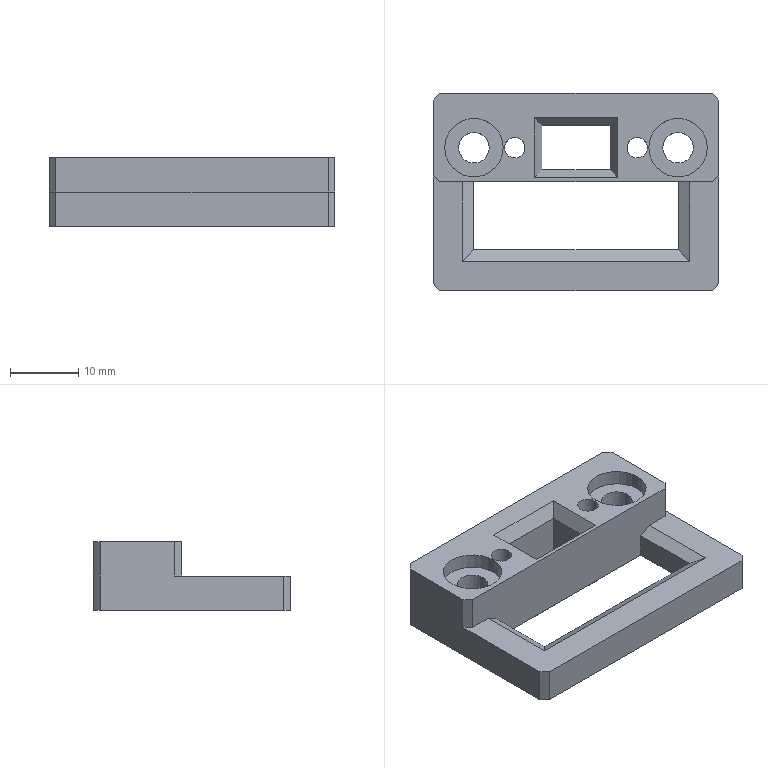Part | NX | features BREP 1 | 1 solid | 50 faces | box 42 x 29 x 10 mm | volume 5876 mm3 | plane 38 | cylinder 12 | commonest cylinder face diameters 3 x4 4.5 x4 8.6 x4
STEP:
#1=CARTESIAN_POINT('',(7.5,0.,-10.));
#2=VERTEX_POINT('',#1);
#3=CARTESIAN_POINT('',(10.5,0.,-10.));
#4=VERTEX_POINT('',#3);
#5=CARTESIAN_POINT('',(9.,0.,-10.));
#6=DIRECTION('',(0.,0.,1.));
#7=DIRECTION('',(1.,0.,0.));
#8=AXIS2_PLACEMENT_3D('',#5,#6,#7);
#9=CIRCLE('',#8,1.5);
#10=EDGE_CURVE('',#2,#4,#9,.T.);
#11=ORIENTED_EDGE('',*,*,#10,.F.);
#12=CARTESIAN_POINT('',(7.5,0.,0.));
#13=VERTEX_POINT('',#12);
#14=CARTESIAN_POINT('',(7.5,0.,-19.));
#15=DIRECTION('',(0.,0.,1.));
#16=VECTOR('',#15,1000.);
#17=LINE('',#14,#16);
#18=EDGE_CURVE('',#13,#2,#17,.F.);
#19=ORIENTED_EDGE('',*,*,#18,.F.);
#20=CARTESIAN_POINT('',(10.5,0.,0.));
#21=VERTEX_POINT('',#20);
#22=CARTESIAN_POINT('',(9.,0.,0.));
#23=DIRECTION('',(0.,0.,1.));
#24=DIRECTION('',(1.,0.,0.));
#25=AXIS2_PLACEMENT_3D('',#22,#23,#24);
#26=CIRCLE('',#25,1.5);
#27=EDGE_CURVE('',#13,#21,#26,.T.);
#28=ORIENTED_EDGE('',*,*,#27,.T.);
#29=CARTESIAN_POINT('',(10.5,0.,-19.));
#30=DIRECTION('',(0.,0.,1.));
#31=VECTOR('',#30,1000.);
#32=LINE('',#29,#31);
#33=EDGE_CURVE('',#21,#4,#32,.F.);
#34=ORIENTED_EDGE('',*,*,#33,.T.);
#35=EDGE_LOOP('',(#11,#19,#28,#34));
#36=FACE_BOUND('',#35,.T.);
#37=CARTESIAN_POINT('',(9.,0.,-19.));
#38=DIRECTION('',(0.,0.,1.));
#39=DIRECTION('',(1.,0.,0.));
#40=AXIS2_PLACEMENT_3D('',#37,#38,#39);
#41=CYLINDRICAL_SURFACE('',#40,1.5);
#42=ADVANCED_FACE('',(#36),#41,.F.);
#43=CARTESIAN_POINT('',(-10.5,0.,-10.));
#44=VERTEX_POINT('',#43);
#45=CARTESIAN_POINT('',(-7.5,0.,-10.));
#46=VERTEX_POINT('',#45);
#47=CARTESIAN_POINT('',(-9.,0.,-10.));
#48=DIRECTION('',(0.,0.,1.));
#49=DIRECTION('',(1.,0.,0.));
#50=AXIS2_PLACEMENT_3D('',#47,#48,#49);
#51=CIRCLE('',#50,1.5);
#52=EDGE_CURVE('',#44,#46,#51,.T.);
#53=ORIENTED_EDGE('',*,*,#52,.F.);
#54=CARTESIAN_POINT('',(-10.5,0.,0.));
#55=VERTEX_POINT('',#54);
#56=CARTESIAN_POINT('',(-10.5,0.,-19.));
#57=DIRECTION('',(0.,0.,1.));
#58=VECTOR('',#57,1000.);
#59=LINE('',#56,#58);
#60=EDGE_CURVE('',#55,#44,#59,.F.);
#61=ORIENTED_EDGE('',*,*,#60,.F.);
#62=CARTESIAN_POINT('',(-7.5,0.,0.));
#63=VERTEX_POINT('',#62);
#64=CARTESIAN_POINT('',(-9.,0.,0.));
#65=DIRECTION('',(0.,0.,1.));
#66=DIRECTION('',(1.,0.,0.));
#67=AXIS2_PLACEMENT_3D('',#64,#65,#66);
#68=CIRCLE('',#67,1.5);
#69=EDGE_CURVE('',#55,#63,#68,.T.);
#70=ORIENTED_EDGE('',*,*,#69,.T.);
#71=CARTESIAN_POINT('',(-7.5,0.,-19.));
#72=DIRECTION('',(0.,0.,1.));
#73=VECTOR('',#72,1000.);
#74=LINE('',#71,#73);
#75=EDGE_CURVE('',#63,#46,#74,.F.);
#76=ORIENTED_EDGE('',*,*,#75,.T.);
#77=EDGE_LOOP('',(#53,#61,#70,#76));
#78=FACE_BOUND('',#77,.T.);
#79=CARTESIAN_POINT('',(-9.,0.,-19.));
#80=DIRECTION('',(0.,0.,1.));
#81=DIRECTION('',(1.,0.,0.));
#82=AXIS2_PLACEMENT_3D('',#79,#80,#81);
#83=CYLINDRICAL_SURFACE('',#82,1.5);
#84=ADVANCED_FACE('',(#78),#83,.F.);
#85=CARTESIAN_POINT('',(-19.3,0.,-2.2));
#86=VERTEX_POINT('',#85);
#87=CARTESIAN_POINT('',(-10.7,0.,-2.2));
#88=VERTEX_POINT('',#87);
#89=CARTESIAN_POINT('',(-15.,0.,-2.2));
#90=DIRECTION('',(0.,0.,1.));
#91=DIRECTION('',(1.,0.,0.));
#92=AXIS2_PLACEMENT_3D('',#89,#90,#91);
#93=CIRCLE('',#92,4.3);
#94=EDGE_CURVE('',#86,#88,#93,.T.);
#95=ORIENTED_EDGE('',*,*,#94,.F.);
#96=CARTESIAN_POINT('',(-19.3,0.,0.));
#97=VERTEX_POINT('',#96);
#98=CARTESIAN_POINT('',(-19.3,0.,0.));
#99=DIRECTION('',(0.,0.,1.));
#100=VECTOR('',#99,1000.);
#101=LINE('',#98,#100);
#102=EDGE_CURVE('',#97,#86,#101,.F.);
#103=ORIENTED_EDGE('',*,*,#102,.F.);
#104=CARTESIAN_POINT('',(-10.7,0.,0.));
#105=VERTEX_POINT('',#104);
#106=CARTESIAN_POINT('',(-15.,0.,0.));
#107=DIRECTION('',(0.,0.,1.));
#108=DIRECTION('',(1.,0.,0.));
#109=AXIS2_PLACEMENT_3D('',#106,#107,#108);
#110=CIRCLE('',#109,4.3);
#111=EDGE_CURVE('',#97,#105,#110,.T.);
#112=ORIENTED_EDGE('',*,*,#111,.T.);
#113=CARTESIAN_POINT('',(-10.7,0.,0.));
#114=DIRECTION('',(0.,0.,1.));
#115=VECTOR('',#114,1000.);
#116=LINE('',#113,#115);
#117=EDGE_CURVE('',#105,#88,#116,.F.);
#118=ORIENTED_EDGE('',*,*,#117,.T.);
#119=EDGE_LOOP('',(#95,#103,#112,#118));
#120=FACE_BOUND('',#119,.T.);
#121=CARTESIAN_POINT('',(-15.,0.,0.));
#122=DIRECTION('',(0.,0.,1.));
#123=DIRECTION('',(1.,0.,0.));
#124=AXIS2_PLACEMENT_3D('',#121,#122,#123);
#125=CYLINDRICAL_SURFACE('',#124,4.3);
#126=ADVANCED_FACE('',(#120),#125,.F.);
#127=CARTESIAN_POINT('',(-17.25,0.,-10.));
#128=VERTEX_POINT('',#127);
#129=CARTESIAN_POINT('',(-12.75,0.,-10.));
#130=VERTEX_POINT('',#129);
#131=CARTESIAN_POINT('',(-15.,0.,-10.));
#132=DIRECTION('',(0.,0.,1.));
#133=DIRECTION('',(1.,0.,0.));
#134=AXIS2_PLACEMENT_3D('',#131,#132,#133);
#135=CIRCLE('',#134,2.25);
#136=EDGE_CURVE('',#128,#130,#135,.T.);
#137=ORIENTED_EDGE('',*,*,#136,.F.);
#138=CARTESIAN_POINT('',(-17.25,0.,-2.2));
#139=VERTEX_POINT('',#138);
#140=CARTESIAN_POINT('',(-17.25,0.,0.));
#141=DIRECTION('',(0.,0.,1.));
#142=VECTOR('',#141,1000.);
#143=LINE('',#140,#142);
#144=EDGE_CURVE('',#139,#128,#143,.F.);
#145=ORIENTED_EDGE('',*,*,#144,.F.);
#146=CARTESIAN_POINT('',(-12.75,0.,-2.2));
#147=VERTEX_POINT('',#146);
#148=CARTESIAN_POINT('',(-15.,0.,-2.2));
#149=DIRECTION('',(0.,0.,1.));
#150=DIRECTION('',(1.,0.,0.));
#151=AXIS2_PLACEMENT_3D('',#148,#149,#150);
#152=CIRCLE('',#151,2.25);
#153=EDGE_CURVE('',#139,#147,#152,.T.);
#154=ORIENTED_EDGE('',*,*,#153,.T.);
#155=CARTESIAN_POINT('',(-12.75,0.,0.));
#156=DIRECTION('',(0.,0.,1.));
#157=VECTOR('',#156,1000.);
#158=LINE('',#155,#157);
#159=EDGE_CURVE('',#147,#130,#158,.F.);
#160=ORIENTED_EDGE('',*,*,#159,.T.);
#161=EDGE_LOOP('',(#137,#145,#154,#160));
#162=FACE_BOUND('',#161,.T.);
#163=CARTESIAN_POINT('',(-15.,0.,0.));
#164=DIRECTION('',(0.,0.,1.));
#165=DIRECTION('',(1.,0.,0.));
#166=AXIS2_PLACEMENT_3D('',#163,#164,#165);
#167=CYLINDRICAL_SURFACE('',#166,2.25);
#168=ADVANCED_FACE('',(#162),#167,.F.);
#169=CARTESIAN_POINT('',(10.7,0.,-2.2));
#170=VERTEX_POINT('',#169);
#171=CARTESIAN_POINT('',(19.3,0.,-2.2));
#172=VERTEX_POINT('',#171);
#173=CARTESIAN_POINT('',(15.,0.,-2.2));
#174=DIRECTION('',(0.,0.,1.));
#175=DIRECTION('',(1.,0.,0.));
#176=AXIS2_PLACEMENT_3D('',#173,#174,#175);
#177=CIRCLE('',#176,4.3);
#178=EDGE_CURVE('',#170,#172,#177,.T.);
#179=ORIENTED_EDGE('',*,*,#178,.F.);
#180=CARTESIAN_POINT('',(10.7,0.,0.));
#181=VERTEX_POINT('',#180);
#182=CARTESIAN_POINT('',(10.7,0.,0.));
#183=DIRECTION('',(0.,0.,1.));
#184=VECTOR('',#183,1000.);
#185=LINE('',#182,#184);
#186=EDGE_CURVE('',#181,#170,#185,.F.);
#187=ORIENTED_EDGE('',*,*,#186,.F.);
#188=CARTESIAN_POINT('',(19.3,0.,0.));
#189=VERTEX_POINT('',#188);
#190=CARTESIAN_POINT('',(15.,0.,0.));
#191=DIRECTION('',(0.,0.,1.));
#192=DIRECTION('',(1.,0.,0.));
#193=AXIS2_PLACEMENT_3D('',#190,#191,#192);
#194=CIRCLE('',#193,4.3);
#195=EDGE_CURVE('',#181,#189,#194,.T.);
#196=ORIENTED_EDGE('',*,*,#195,.T.);
#197=CARTESIAN_POINT('',(19.3,0.,0.));
#198=DIRECTION('',(0.,0.,1.));
#199=VECTOR('',#198,1000.);
#200=LINE('',#197,#199);
#201=EDGE_CURVE('',#189,#172,#200,.F.);
#202=ORIENTED_EDGE('',*,*,#201,.T.);
#203=EDGE_LOOP('',(#179,#187,#196,#202));
#204=FACE_BOUND('',#203,.T.);
#205=CARTESIAN_POINT('',(15.,0.,0.));
#206=DIRECTION('',(0.,0.,1.));
#207=DIRECTION('',(1.,0.,0.));
#208=AXIS2_PLACEMENT_3D('',#205,#206,#207);
#209=CYLINDRICAL_SURFACE('',#208,4.3);
#210=ADVANCED_FACE('',(#204),#209,.F.);
#211=CARTESIAN_POINT('',(12.75,0.,-10.));
#212=VERTEX_POINT('',#211);
#213=CARTESIAN_POINT('',(17.25,0.,-10.));
#214=VERTEX_POINT('',#213);
#215=CARTESIAN_POINT('',(15.,0.,-10.));
#216=DIRECTION('',(0.,0.,1.));
#217=DIRECTION('',(1.,0.,0.));
#218=AXIS2_PLACEMENT_3D('',#215,#216,#217);
#219=CIRCLE('',#218,2.25);
#220=EDGE_CURVE('',#212,#214,#219,.T.);
#221=ORIENTED_EDGE('',*,*,#220,.F.);
#222=CARTESIAN_POINT('',(12.75,0.,-2.2));
#223=VERTEX_POINT('',#222);
#224=CARTESIAN_POINT('',(12.75,0.,0.));
#225=DIRECTION('',(0.,0.,1.));
#226=VECTOR('',#225,1000.);
#227=LINE('',#224,#226);
#228=EDGE_CURVE('',#223,#212,#227,.F.);
#229=ORIENTED_EDGE('',*,*,#228,.F.);
#230=CARTESIAN_POINT('',(17.25,0.,-2.2));
#231=VERTEX_POINT('',#230);
#232=CARTESIAN_POINT('',(15.,0.,-2.2));
#233=DIRECTION('',(0.,0.,1.));
#234=DIRECTION('',(1.,0.,0.));
#235=AXIS2_PLACEMENT_3D('',#232,#233,#234);
#236=CIRCLE('',#235,2.25);
#237=EDGE_CURVE('',#223,#231,#236,.T.);
#238=ORIENTED_EDGE('',*,*,#237,.T.);
#239=CARTESIAN_POINT('',(17.25,0.,0.));
#240=DIRECTION('',(0.,0.,1.));
#241=VECTOR('',#240,1000.);
#242=LINE('',#239,#241);
#243=EDGE_CURVE('',#231,#214,#242,.F.);
#244=ORIENTED_EDGE('',*,*,#243,.T.);
#245=EDGE_LOOP('',(#221,#229,#238,#244));
#246=FACE_BOUND('',#245,.T.);
#247=CARTESIAN_POINT('',(15.,0.,0.));
#248=DIRECTION('',(0.,0.,1.));
#249=DIRECTION('',(1.,0.,0.));
#250=AXIS2_PLACEMENT_3D('',#247,#248,#249);
#251=CYLINDRICAL_SURFACE('',#250,2.25);
#252=ADVANCED_FACE('',(#246),#251,.F.);
#253=CARTESIAN_POINT('',(-20.,-21.,-5.));
#254=VERTEX_POINT('',#253);
#255=CARTESIAN_POINT('',(20.,-21.,-5.));
#256=VERTEX_POINT('',#255);
#257=CARTESIAN_POINT('',(-21.,-21.,-5.));
#258=DIRECTION('',(1.,0.,0.));
#259=VECTOR('',#258,1000.);
#260=LINE('',#257,#259);
#261=EDGE_CURVE('',#254,#256,#260,.T.);
#262=ORIENTED_EDGE('',*,*,#261,.F.);
#263=CARTESIAN_POINT('',(-20.,-21.,-10.));
#264=VERTEX_POINT('',#263);
#265=CARTESIAN_POINT('',(-20.,-21.,0.));
#266=DIRECTION('',(0.,0.,-1.));
#267=VECTOR('',#266,1000.);
#268=LINE('',#265,#267);
#269=EDGE_CURVE('',#254,#264,#268,.T.);
#270=ORIENTED_EDGE('',*,*,#269,.T.);
#271=CARTESIAN_POINT('',(20.,-21.,-10.));
#272=VERTEX_POINT('',#271);
#273=CARTESIAN_POINT('',(-21.,-21.,-10.));
#274=DIRECTION('',(1.,0.,0.));
#275=VECTOR('',#274,1000.);
#276=LINE('',#273,#275);
#277=EDGE_CURVE('',#264,#272,#276,.T.);
#278=ORIENTED_EDGE('',*,*,#277,.T.);
#279=CARTESIAN_POINT('',(20.,-21.,0.));
#280=DIRECTION('',(0.,0.,1.));
#281=VECTOR('',#280,1000.);
#282=LINE('',#279,#281);
#283=EDGE_CURVE('',#272,#256,#282,.T.);
#284=ORIENTED_EDGE('',*,*,#283,.T.);
#285=EDGE_LOOP('',(#262,#270,#278,#284));
#286=FACE_BOUND('',#285,.T.);
#287=CARTESIAN_POINT('',(0.,-21.,0.));
#288=DIRECTION('',(0.,-1.,0.));
#289=DIRECTION('',(0.,0.,-1.));
#290=AXIS2_PLACEMENT_3D('',#287,#288,#289);
#291=PLANE('',#290);
#292=ADVANCED_FACE('',(#286),#291,.T.);
#293=CARTESIAN_POINT('',(15.,-15.,-9.5));
#294=VERTEX_POINT('',#293);
#295=CARTESIAN_POINT('',(15.,-15.,-6.));
#296=VERTEX_POINT('',#295);
#297=CARTESIAN_POINT('',(15.,-15.,-16.));
#298=DIRECTION('',(0.,0.,1.));
#299=VECTOR('',#298,1000.);
#300=LINE('',#297,#299);
#301=EDGE_CURVE('',#294,#296,#300,.T.);
#302=ORIENTED_EDGE('',*,*,#301,.T.);
#303=CARTESIAN_POINT('',(15.,-5.,-6.));
#304=VERTEX_POINT('',#303);
#305=CARTESIAN_POINT('',(15.,-5.,-6.));
#306=DIRECTION('',(0.,1.,0.));
#307=VECTOR('',#306,1000.);
#308=LINE('',#305,#307);
#309=EDGE_CURVE('',#296,#304,#308,.T.);
#310=ORIENTED_EDGE('',*,*,#309,.T.);
#311=CARTESIAN_POINT('',(15.,-5.,-9.5));
#312=VERTEX_POINT('',#311);
#313=CARTESIAN_POINT('',(15.,-5.,-16.));
#314=DIRECTION('',(0.,0.,1.));
#315=VECTOR('',#314,1000.);
#316=LINE('',#313,#315);
#317=EDGE_CURVE('',#312,#304,#316,.T.);
#318=ORIENTED_EDGE('',*,*,#317,.F.);
#319=CARTESIAN_POINT('',(15.,-15.,-9.5));
#320=DIRECTION('',(0.,-1.,0.));
#321=VECTOR('',#320,1000.);
#322=LINE('',#319,#321);
#323=EDGE_CURVE('',#312,#294,#322,.T.);
#324=ORIENTED_EDGE('',*,*,#323,.T.);
#325=EDGE_LOOP('',(#302,#310,#318,#324));
#326=FACE_BOUND('',#325,.T.);
#327=CARTESIAN_POINT('',(15.,-15.,-16.));
#328=DIRECTION('',(1.,0.,0.));
#329=DIRECTION('',(0.,1.,0.));
#330=AXIS2_PLACEMENT_3D('',#327,#328,#329);
#331=PLANE('',#330);
#332=ADVANCED_FACE('',(#326),#331,.F.);
#333=CARTESIAN_POINT('',(-15.,-15.,-9.5));
#334=VERTEX_POINT('',#333);
#335=CARTESIAN_POINT('',(-15.,-15.,-6.));
#336=VERTEX_POINT('',#335);
#337=CARTESIAN_POINT('',(-15.,-15.,-16.));
#338=DIRECTION('',(0.,0.,1.));
#339=VECTOR('',#338,1000.);
#340=LINE('',#337,#339);
#341=EDGE_CURVE('',#334,#336,#340,.T.);
#342=ORIENTED_EDGE('',*,*,#341,.T.);
#343=CARTESIAN_POINT('',(15.,-15.,-6.));
#344=DIRECTION('',(1.,0.,0.));
#345=VECTOR('',#344,1000.);
#346=LINE('',#343,#345);
#347=EDGE_CURVE('',#336,#296,#346,.T.);
#348=ORIENTED_EDGE('',*,*,#347,.T.);
#349=ORIENTED_EDGE('',*,*,#301,.F.);
#350=CARTESIAN_POINT('',(15.,-15.,-9.5));
#351=DIRECTION('',(-1.,0.,0.));
#352=VECTOR('',#351,1000.);
#353=LINE('',#350,#352);
#354=EDGE_CURVE('',#294,#334,#353,.T.);
#355=ORIENTED_EDGE('',*,*,#354,.T.);
#356=EDGE_LOOP('',(#342,#348,#349,#355));
#357=FACE_BOUND('',#356,.T.);
#358=CARTESIAN_POINT('',(15.,-15.,-16.));
#359=DIRECTION('',(0.,-1.,0.));
#360=DIRECTION('',(0.,0.,-1.));
#361=AXIS2_PLACEMENT_3D('',#358,#359,#360);
#362=PLANE('',#361);
#363=ADVANCED_FACE('',(#357),#362,.F.);
#364=CARTESIAN_POINT('',(-15.,-5.,-9.5));
#365=VERTEX_POINT('',#364);
#366=CARTESIAN_POINT('',(-15.,-5.,-6.));
#367=VERTEX_POINT('',#366);
#368=CARTESIAN_POINT('',(-15.,-5.,-16.));
#369=DIRECTION('',(0.,0.,1.));
#370=VECTOR('',#369,1000.);
#371=LINE('',#368,#370);
#372=EDGE_CURVE('',#365,#367,#371,.T.);
#373=ORIENTED_EDGE('',*,*,#372,.T.);
#374=CARTESIAN_POINT('',(-15.,-15.,-6.));
#375=DIRECTION('',(0.,-1.,0.));
#376=VECTOR('',#375,1000.);
#377=LINE('',#374,#376);
#378=EDGE_CURVE('',#367,#336,#377,.T.);
#379=ORIENTED_EDGE('',*,*,#378,.T.);
#380=ORIENTED_EDGE('',*,*,#341,.F.);
#381=CARTESIAN_POINT('',(-15.,-15.,-9.5));
#382=DIRECTION('',(0.,1.,0.));
#383=VECTOR('',#382,1000.);
#384=LINE('',#381,#383);
#385=EDGE_CURVE('',#334,#365,#384,.T.);
#386=ORIENTED_EDGE('',*,*,#385,.T.);
#387=EDGE_LOOP('',(#373,#379,#380,#386));
#388=FACE_BOUND('',#387,.T.);
#389=CARTESIAN_POINT('',(-15.,-15.,-16.));
#390=DIRECTION('',(-1.,0.,0.));
#391=DIRECTION('',(0.,0.,1.));
#392=AXIS2_PLACEMENT_3D('',#389,#390,#391);
#393=PLANE('',#392);
#394=ADVANCED_FACE('',(#388),#393,.F.);
#395=CARTESIAN_POINT('',(21.,-4.,0.));
#396=VERTEX_POINT('',#395);
#397=CARTESIAN_POINT('',(21.,7.,0.));
#398=VERTEX_POINT('',#397);
#399=CARTESIAN_POINT('',(21.,5.,0.));
#400=DIRECTION('',(0.,1.,0.));
#401=VECTOR('',#400,1000.);
#402=LINE('',#399,#401);
#403=EDGE_CURVE('',#396,#398,#402,.T.);
#404=ORIENTED_EDGE('',*,*,#403,.F.);
#405=CARTESIAN_POINT('',(21.,-4.,-5.));
#406=VERTEX_POINT('',#405);
#407=CARTESIAN_POINT('',(21.,-4.,-5.));
#408=DIRECTION('',(0.,0.,-1.));
#409=VECTOR('',#408,1000.);
#410=LINE('',#407,#409);
#411=EDGE_CURVE('',#396,#406,#410,.T.);
#412=ORIENTED_EDGE('',*,*,#411,.T.);
#413=CARTESIAN_POINT('',(21.,-20.,-5.));
#414=VERTEX_POINT('',#413);
#415=CARTESIAN_POINT('',(21.,-5.,-5.));
#416=DIRECTION('',(0.,1.,0.));
#417=VECTOR('',#416,1000.);
#418=LINE('',#415,#417);
#419=EDGE_CURVE('',#414,#406,#418,.T.);
#420=ORIENTED_EDGE('',*,*,#419,.F.);
#421=CARTESIAN_POINT('',(21.,-20.,-10.));
#422=VERTEX_POINT('',#421);
#423=CARTESIAN_POINT('',(21.,-20.,-10.));
#424=DIRECTION('',(0.,0.,-1.));
#425=VECTOR('',#424,1000.);
#426=LINE('',#423,#425);
#427=EDGE_CURVE('',#414,#422,#426,.T.);
#428=ORIENTED_EDGE('',*,*,#427,.T.);
#429=CARTESIAN_POINT('',(21.,7.,-10.));
#430=VERTEX_POINT('',#429);
#431=CARTESIAN_POINT('',(21.,5.,-10.));
#432=DIRECTION('',(0.,1.,0.));
#433=VECTOR('',#432,1000.);
#434=LINE('',#431,#433);
#435=EDGE_CURVE('',#422,#430,#434,.T.);
#436=ORIENTED_EDGE('',*,*,#435,.T.);
#437=CARTESIAN_POINT('',(21.,7.,-10.));
#438=DIRECTION('',(0.,0.,1.));
#439=VECTOR('',#438,1000.);
#440=LINE('',#437,#439);
#441=EDGE_CURVE('',#430,#398,#440,.T.);
#442=ORIENTED_EDGE('',*,*,#441,.T.);
#443=EDGE_LOOP('',(#404,#412,#420,#428,#436,#442));
#444=FACE_BOUND('',#443,.T.);
#445=CARTESIAN_POINT('',(21.,5.,-10.));
#446=DIRECTION('',(1.,0.,0.));
#447=DIRECTION('',(0.,1.,0.));
#448=AXIS2_PLACEMENT_3D('',#445,#446,#447);
#449=PLANE('',#448);
#450=ADVANCED_FACE('',(#444),#449,.T.);
#451=CARTESIAN_POINT('',(-21.,-4.,-5.));
#452=VERTEX_POINT('',#451);
#453=CARTESIAN_POINT('',(-21.,-20.,-5.));
#454=VERTEX_POINT('',#453);
#455=CARTESIAN_POINT('',(-21.,-5.,-5.));
#456=DIRECTION('',(0.,-1.,0.));
#457=VECTOR('',#456,1000.);
#458=LINE('',#455,#457);
#459=EDGE_CURVE('',#452,#454,#458,.T.);
#460=ORIENTED_EDGE('',*,*,#459,.F.);
#461=CARTESIAN_POINT('',(-21.,-4.,0.));
#462=VERTEX_POINT('',#461);
#463=CARTESIAN_POINT('',(-21.,-4.,0.));
#464=DIRECTION('',(0.,0.,1.));
#465=VECTOR('',#464,1000.);
#466=LINE('',#463,#465);
#467=EDGE_CURVE('',#452,#462,#466,.T.);
#468=ORIENTED_EDGE('',*,*,#467,.T.);
#469=CARTESIAN_POINT('',(-21.,7.,0.));
#470=VERTEX_POINT('',#469);
#471=CARTESIAN_POINT('',(-21.,5.,0.));
#472=DIRECTION('',(0.,-1.,0.));
#473=VECTOR('',#472,1000.);
#474=LINE('',#471,#473);
#475=EDGE_CURVE('',#470,#462,#474,.T.);
#476=ORIENTED_EDGE('',*,*,#475,.F.);
#477=CARTESIAN_POINT('',(-21.,7.,-10.));
#478=VERTEX_POINT('',#477);
#479=CARTESIAN_POINT('',(-21.,7.,-10.));
#480=DIRECTION('',(0.,0.,-1.));
#481=VECTOR('',#480,1000.);
#482=LINE('',#479,#481);
#483=EDGE_CURVE('',#470,#478,#482,.T.);
#484=ORIENTED_EDGE('',*,*,#483,.T.);
#485=CARTESIAN_POINT('',(-21.,-20.,-10.));
#486=VERTEX_POINT('',#485);
#487=CARTESIAN_POINT('',(-21.,5.,-10.));
#488=DIRECTION('',(0.,-1.,0.));
#489=VECTOR('',#488,1000.);
#490=LINE('',#487,#489);
#491=EDGE_CURVE('',#478,#486,#490,.T.);
#492=ORIENTED_EDGE('',*,*,#491,.T.);
#493=CARTESIAN_POINT('',(-21.,-20.,-10.));
#494=DIRECTION('',(0.,0.,1.));
#495=VECTOR('',#494,1000.);
#496=LINE('',#493,#495);
#497=EDGE_CURVE('',#486,#454,#496,.T.);
#498=ORIENTED_EDGE('',*,*,#497,.T.);
#499=EDGE_LOOP('',(#460,#468,#476,#484,#492,#498));
#500=FACE_BOUND('',#499,.T.);
#501=CARTESIAN_POINT('',(-21.,5.,-10.));
#502=DIRECTION('',(-1.,0.,0.));
#503=DIRECTION('',(0.,1.,0.));
#504=AXIS2_PLACEMENT_3D('',#501,#502,#503);
#505=PLANE('',#504);
#506=ADVANCED_FACE('',(#500),#505,.T.);
#507=ORIENTED_EDGE('',*,*,#277,.F.);
#508=CARTESIAN_POINT('',(-20.,-21.,-10.));
#509=DIRECTION('',(-0.7071,0.7071,0.));
#510=VECTOR('',#509,1000.);
#511=LINE('',#508,#510);
#512=EDGE_CURVE('',#264,#486,#511,.T.);
#513=ORIENTED_EDGE('',*,*,#512,.T.);
#514=ORIENTED_EDGE('',*,*,#491,.F.);
#515=CARTESIAN_POINT('',(-20.,8.,-10.));
#516=VERTEX_POINT('',#515);
#517=CARTESIAN_POINT('',(-20.,8.,-10.));
#518=DIRECTION('',(0.7071,0.7071,0.));
#519=VECTOR('',#518,1000.);
#520=LINE('',#517,#519);
#521=EDGE_CURVE('',#478,#516,#520,.T.);
#522=ORIENTED_EDGE('',*,*,#521,.T.);
#523=CARTESIAN_POINT('',(20.,8.,-10.));
#524=VERTEX_POINT('',#523);
#525=CARTESIAN_POINT('',(-21.,8.,-10.));
#526=DIRECTION('',(-1.,0.,0.));
#527=VECTOR('',#526,1000.);
#528=LINE('',#525,#527);
#529=EDGE_CURVE('',#524,#516,#528,.T.);
#530=ORIENTED_EDGE('',*,*,#529,.F.);
#531=CARTESIAN_POINT('',(20.,8.,-10.));
#532=DIRECTION('',(0.7071,-0.7071,0.));
#533=VECTOR('',#532,1000.);
#534=LINE('',#531,#533);
#535=EDGE_CURVE('',#524,#430,#534,.T.);
#536=ORIENTED_EDGE('',*,*,#535,.T.);
#537=ORIENTED_EDGE('',*,*,#435,.F.);
#538=CARTESIAN_POINT('',(20.,-21.,-10.));
#539=DIRECTION('',(-0.7071,-0.7071,0.));
#540=VECTOR('',#539,1000.);
#541=LINE('',#538,#540);
#542=EDGE_CURVE('',#422,#272,#541,.T.);
#543=ORIENTED_EDGE('',*,*,#542,.T.);
#544=EDGE_LOOP('',(#507,#513,#514,#522,#530,#536,#537,#543));
#545=FACE_BOUND('',#544,.T.);
#546=CARTESIAN_POINT('',(15.5,-4.5,-10.));
#547=VERTEX_POINT('',#546);
#548=CARTESIAN_POINT('',(6.732,-4.5,-10.));
#549=VERTEX_POINT('',#548);
#550=CARTESIAN_POINT('',(0.,-4.5,-10.));
#551=DIRECTION('',(-1.,0.,0.));
#552=VECTOR('',#551,1000.);
#553=LINE('',#550,#552);
#554=EDGE_CURVE('',#547,#549,#553,.T.);
#555=ORIENTED_EDGE('',*,*,#554,.T.);
#556=CARTESIAN_POINT('',(6.732,4.982,-10.));
#557=VERTEX_POINT('',#556);
#558=CARTESIAN_POINT('',(6.732,0.,-10.));
#559=DIRECTION('',(0.,1.,0.));
#560=VECTOR('',#559,1000.);
#561=LINE('',#558,#560);
#562=EDGE_CURVE('',#549,#557,#561,.T.);
#563=ORIENTED_EDGE('',*,*,#562,.T.);
#564=CARTESIAN_POINT('',(-6.732,4.982,-10.));
#565=VERTEX_POINT('',#564);
#566=CARTESIAN_POINT('',(0.,4.982,-10.));
#567=DIRECTION('',(-1.,0.,0.));
#568=VECTOR('',#567,1000.);
#569=LINE('',#566,#568);
#570=EDGE_CURVE('',#557,#565,#569,.T.);
#571=ORIENTED_EDGE('',*,*,#570,.T.);
#572=CARTESIAN_POINT('',(-6.732,-4.5,-10.));
#573=VERTEX_POINT('',#572);
#574=CARTESIAN_POINT('',(-6.732,0.,-10.));
#575=DIRECTION('',(0.,-1.,0.));
#576=VECTOR('',#575,1000.);
#577=LINE('',#574,#576);
#578=EDGE_CURVE('',#565,#573,#577,.T.);
#579=ORIENTED_EDGE('',*,*,#578,.T.);
#580=CARTESIAN_POINT('',(-15.5,-4.5,-10.));
#581=VERTEX_POINT('',#580);
#582=CARTESIAN_POINT('',(0.,-4.5,-10.));
#583=DIRECTION('',(-1.,0.,0.));
#584=VECTOR('',#583,1000.);
#585=LINE('',#582,#584);
#586=EDGE_CURVE('',#573,#581,#585,.T.);
#587=ORIENTED_EDGE('',*,*,#586,.T.);
#588=CARTESIAN_POINT('',(-15.5,-15.5,-10.));
#589=VERTEX_POINT('',#588);
#590=CARTESIAN_POINT('',(-15.5,0.,-10.));
#591=DIRECTION('',(0.,-1.,0.));
#592=VECTOR('',#591,1000.);
#593=LINE('',#590,#592);
#594=EDGE_CURVE('',#581,#589,#593,.T.);
#595=ORIENTED_EDGE('',*,*,#594,.T.);
#596=CARTESIAN_POINT('',(15.5,-15.5,-10.));
#597=VERTEX_POINT('',#596);
#598=CARTESIAN_POINT('',(0.,-15.5,-10.));
#599=DIRECTION('',(1.,0.,0.));
#600=VECTOR('',#599,1000.);
#601=LINE('',#598,#600);
#602=EDGE_CURVE('',#589,#597,#601,.T.);
#603=ORIENTED_EDGE('',*,*,#602,.T.);
#604=CARTESIAN_POINT('',(15.5,0.,-10.));
#605=DIRECTION('',(0.,1.,0.));
#606=VECTOR('',#605,1000.);
#607=LINE('',#604,#606);
#608=EDGE_CURVE('',#597,#547,#607,.T.);
#609=ORIENTED_EDGE('',*,*,#608,.T.);
#610=EDGE_LOOP('',(#555,#563,#571,#579,#587,#595,#603,#609));
#611=FACE_BOUND('',#610,.T.);
#612=CARTESIAN_POINT('',(9.,0.,-10.));
#613=DIRECTION('',(0.,0.,1.));
#614=DIRECTION('',(1.,0.,0.));
#615=AXIS2_PLACEMENT_3D('',#612,#613,#614);
#616=CIRCLE('',#615,1.5);
#617=EDGE_CURVE('',#4,#2,#616,.T.);
#618=ORIENTED_EDGE('',*,*,#617,.T.);
#619=ORIENTED_EDGE('',*,*,#10,.T.);
#620=EDGE_LOOP('',(#618,#619));
#621=FACE_BOUND('',#620,.T.);
#622=CARTESIAN_POINT('',(-9.,0.,-10.));
#623=DIRECTION('',(0.,0.,1.));
#624=DIRECTION('',(1.,0.,0.));
#625=AXIS2_PLACEMENT_3D('',#622,#623,#624);
#626=CIRCLE('',#625,1.5);
#627=EDGE_CURVE('',#46,#44,#626,.T.);
#628=ORIENTED_EDGE('',*,*,#627,.T.);
#629=ORIENTED_EDGE('',*,*,#52,.T.);
#630=EDGE_LOOP('',(#628,#629));
#631=FACE_BOUND('',#630,.T.);
#632=CARTESIAN_POINT('',(-15.,0.,-10.));
#633=DIRECTION('',(0.,0.,1.));
#634=DIRECTION('',(1.,0.,0.));
#635=AXIS2_PLACEMENT_3D('',#632,#633,#634);
#636=CIRCLE('',#635,2.25);
#637=EDGE_CURVE('',#130,#128,#636,.T.);
#638=ORIENTED_EDGE('',*,*,#637,.T.);
#639=ORIENTED_EDGE('',*,*,#136,.T.);
#640=EDGE_LOOP('',(#638,#639));
#641=FACE_BOUND('',#640,.T.);
#642=CARTESIAN_POINT('',(15.,0.,-10.));
#643=DIRECTION('',(0.,0.,1.));
#644=DIRECTION('',(1.,0.,0.));
#645=AXIS2_PLACEMENT_3D('',#642,#643,#644);
#646=CIRCLE('',#645,2.25);
#647=EDGE_CURVE('',#214,#212,#646,.T.);
#648=ORIENTED_EDGE('',*,*,#647,.T.);
#649=ORIENTED_EDGE('',*,*,#220,.T.);
#650=EDGE_LOOP('',(#648,#649));
#651=FACE_BOUND('',#650,.T.);
#652=CARTESIAN_POINT('',(0.,0.,-10.));
#653=DIRECTION('',(0.,0.,1.));
#654=DIRECTION('',(1.,0.,0.));
#655=AXIS2_PLACEMENT_3D('',#652,#653,#654);
#656=PLANE('',#655);
#657=ADVANCED_FACE('',(#545,#611,#621,#631,#641,#651),#656,.F.);
#658=ORIENTED_EDGE('',*,*,#475,.T.);
#659=CARTESIAN_POINT('',(-20.,-5.,0.));
#660=VERTEX_POINT('',#659);
#661=CARTESIAN_POINT('',(-12.5,-12.5,0.));
#662=DIRECTION('',(0.7071,-0.7071,0.));
#663=VECTOR('',#662,1000.);
#664=LINE('',#661,#663);
#665=EDGE_CURVE('',#462,#660,#664,.T.);
#666=ORIENTED_EDGE('',*,*,#665,.T.);
#667=CARTESIAN_POINT('',(20.,-5.,0.));
#668=VERTEX_POINT('',#667);
#669=CARTESIAN_POINT('',(15.,-5.,0.));
#670=DIRECTION('',(-1.,0.,0.));
#671=VECTOR('',#670,1000.);
#672=LINE('',#669,#671);
#673=EDGE_CURVE('',#668,#660,#672,.T.);
#674=ORIENTED_EDGE('',*,*,#673,.F.);
#675=CARTESIAN_POINT('',(12.5,-12.5,0.));
#676=DIRECTION('',(0.7071,0.7071,0.));
#677=VECTOR('',#676,1000.);
#678=LINE('',#675,#677);
#679=EDGE_CURVE('',#668,#396,#678,.T.);
#680=ORIENTED_EDGE('',*,*,#679,.T.);
#681=ORIENTED_EDGE('',*,*,#403,.T.);
#682=CARTESIAN_POINT('',(20.,8.,0.));
#683=VERTEX_POINT('',#682);
#684=CARTESIAN_POINT('',(14.,14.,0.));
#685=DIRECTION('',(-0.7071,0.7071,0.));
#686=VECTOR('',#685,1000.);
#687=LINE('',#684,#686);
#688=EDGE_CURVE('',#398,#683,#687,.T.);
#689=ORIENTED_EDGE('',*,*,#688,.T.);
#690=CARTESIAN_POINT('',(-20.,8.,0.));
#691=VERTEX_POINT('',#690);
#692=CARTESIAN_POINT('',(-21.,8.,0.));
#693=DIRECTION('',(1.,0.,0.));
#694=VECTOR('',#693,1000.);
#695=LINE('',#692,#694);
#696=EDGE_CURVE('',#691,#683,#695,.T.);
#697=ORIENTED_EDGE('',*,*,#696,.F.);
#698=CARTESIAN_POINT('',(-14.,14.,0.));
#699=DIRECTION('',(-0.7071,-0.7071,0.));
#700=VECTOR('',#699,1000.);
#701=LINE('',#698,#700);
#702=EDGE_CURVE('',#691,#470,#701,.T.);
#703=ORIENTED_EDGE('',*,*,#702,.T.);
#704=EDGE_LOOP('',(#658,#666,#674,#680,#681,#689,#697,#703));
#705=FACE_BOUND('',#704,.T.);
#706=CARTESIAN_POINT('',(9.,0.,0.));
#707=DIRECTION('',(0.,0.,1.));
#708=DIRECTION('',(1.,0.,0.));
#709=AXIS2_PLACEMENT_3D('',#706,#707,#708);
#710=CIRCLE('',#709,1.5);
#711=EDGE_CURVE('',#21,#13,#710,.T.);
#712=ORIENTED_EDGE('',*,*,#711,.F.);
#713=ORIENTED_EDGE('',*,*,#27,.F.);
#714=EDGE_LOOP('',(#712,#713));
#715=FACE_BOUND('',#714,.T.);
#716=CARTESIAN_POINT('',(-9.,0.,0.));
#717=DIRECTION('',(0.,0.,1.));
#718=DIRECTION('',(1.,0.,0.));
#719=AXIS2_PLACEMENT_3D('',#716,#717,#718);
#720=CIRCLE('',#719,1.5);
#721=EDGE_CURVE('',#63,#55,#720,.T.);
#722=ORIENTED_EDGE('',*,*,#721,.F.);
#723=ORIENTED_EDGE('',*,*,#69,.F.);
#724=EDGE_LOOP('',(#722,#723));
#725=FACE_BOUND('',#724,.T.);
#726=CARTESIAN_POINT('',(-15.,0.,0.));
#727=DIRECTION('',(0.,0.,1.));
#728=DIRECTION('',(1.,0.,0.));
#729=AXIS2_PLACEMENT_3D('',#726,#727,#728);
#730=CIRCLE('',#729,4.3);
#731=EDGE_CURVE('',#105,#97,#730,.T.);
#732=ORIENTED_EDGE('',*,*,#731,.F.);
#733=ORIENTED_EDGE('',*,*,#111,.F.);
#734=EDGE_LOOP('',(#732,#733));
#735=FACE_BOUND('',#734,.T.);
#736=CARTESIAN_POINT('',(15.,0.,0.));
#737=DIRECTION('',(0.,0.,1.));
#738=DIRECTION('',(1.,0.,0.));
#739=AXIS2_PLACEMENT_3D('',#736,#737,#738);
#740=CIRCLE('',#739,4.3);
#741=EDGE_CURVE('',#189,#181,#740,.T.);
#742=ORIENTED_EDGE('',*,*,#741,.F.);
#743=ORIENTED_EDGE('',*,*,#195,.F.);
#744=EDGE_LOOP('',(#742,#743));
#745=FACE_BOUND('',#744,.T.);
#746=CARTESIAN_POINT('',(6.155,4.405,0.));
#747=VERTEX_POINT('',#746);
#748=CARTESIAN_POINT('',(6.155,-4.405,0.));
#749=VERTEX_POINT('',#748);
#750=CARTESIAN_POINT('',(6.155,-3.25,0.));
#751=DIRECTION('',(0.,-1.,0.));
#752=VECTOR('',#751,1000.);
#753=LINE('',#750,#752);
#754=EDGE_CURVE('',#747,#749,#753,.T.);
#755=ORIENTED_EDGE('',*,*,#754,.T.);
#756=CARTESIAN_POINT('',(-6.155,-4.405,0.));
#757=VERTEX_POINT('',#756);
#758=CARTESIAN_POINT('',(-5.,-4.405,0.));
#759=DIRECTION('',(-1.,0.,0.));
#760=VECTOR('',#759,1000.);
#761=LINE('',#758,#760);
#762=EDGE_CURVE('',#749,#757,#761,.T.);
#763=ORIENTED_EDGE('',*,*,#762,.T.);
#764=CARTESIAN_POINT('',(-6.155,4.405,0.));
#765=VERTEX_POINT('',#764);
#766=CARTESIAN_POINT('',(-6.155,3.25,0.));
#767=DIRECTION('',(0.,1.,0.));
#768=VECTOR('',#767,1000.);
#769=LINE('',#766,#768);
#770=EDGE_CURVE('',#757,#765,#769,.T.);
#771=ORIENTED_EDGE('',*,*,#770,.T.);
#772=CARTESIAN_POINT('',(5.,4.405,0.));
#773=DIRECTION('',(1.,0.,0.));
#774=VECTOR('',#773,1000.);
#775=LINE('',#772,#774);
#776=EDGE_CURVE('',#765,#747,#775,.T.);
#777=ORIENTED_EDGE('',*,*,#776,.T.);
#778=EDGE_LOOP('',(#755,#763,#771,#777));
#779=FACE_BOUND('',#778,.T.);
#780=CARTESIAN_POINT('',(0.,0.,0.));
#781=DIRECTION('',(0.,0.,1.));
#782=DIRECTION('',(1.,0.,0.));
#783=AXIS2_PLACEMENT_3D('',#780,#781,#782);
#784=PLANE('',#783);
#785=ADVANCED_FACE('',(#705,#715,#725,#735,#745,#779),#784,.T.);
#786=CARTESIAN_POINT('',(5.,3.25,-9.));
#787=VERTEX_POINT('',#786);
#788=CARTESIAN_POINT('',(5.,3.25,-2.));
#789=VERTEX_POINT('',#788);
#790=CARTESIAN_POINT('',(5.,3.25,-24.));
#791=DIRECTION('',(0.,0.,1.));
#792=VECTOR('',#791,1000.);
#793=LINE('',#790,#792);
#794=EDGE_CURVE('',#787,#789,#793,.T.);
#795=ORIENTED_EDGE('',*,*,#794,.F.);
#796=CARTESIAN_POINT('',(5.,-3.25,-9.));
#797=VERTEX_POINT('',#796);
#798=CARTESIAN_POINT('',(5.,3.25,-9.));
#799=DIRECTION('',(0.,-1.,0.));
#800=VECTOR('',#799,1000.);
#801=LINE('',#798,#800);
#802=EDGE_CURVE('',#787,#797,#801,.T.);
#803=ORIENTED_EDGE('',*,*,#802,.T.);
#804=CARTESIAN_POINT('',(5.,-3.25,-2.));
#805=VERTEX_POINT('',#804);
#806=CARTESIAN_POINT('',(5.,-3.25,-24.));
#807=DIRECTION('',(0.,0.,1.));
#808=VECTOR('',#807,1000.);
#809=LINE('',#806,#808);
#810=EDGE_CURVE('',#797,#805,#809,.T.);
#811=ORIENTED_EDGE('',*,*,#810,.T.);
#812=CARTESIAN_POINT('',(5.,3.25,-2.));
#813=DIRECTION('',(0.,1.,0.));
#814=VECTOR('',#813,1000.);
#815=LINE('',#812,#814);
#816=EDGE_CURVE('',#805,#789,#815,.T.);
#817=ORIENTED_EDGE('',*,*,#816,.T.);
#818=EDGE_LOOP('',(#795,#803,#811,#817));
#819=FACE_BOUND('',#818,.T.);
#820=CARTESIAN_POINT('',(5.,3.25,-24.));
#821=DIRECTION('',(1.,0.,0.));
#822=DIRECTION('',(0.,1.,0.));
#823=AXIS2_PLACEMENT_3D('',#820,#821,#822);
#824=PLANE('',#823);
#825=ADVANCED_FACE('',(#819),#824,.F.);
#826=ORIENTED_EDGE('',*,*,#810,.F.);
#827=CARTESIAN_POINT('',(-5.,-3.25,-9.));
#828=VERTEX_POINT('',#827);
#829=CARTESIAN_POINT('',(-5.,-3.25,-9.));
#830=DIRECTION('',(-1.,0.,0.));
#831=VECTOR('',#830,1000.);
#832=LINE('',#829,#831);
#833=EDGE_CURVE('',#797,#828,#832,.T.);
#834=ORIENTED_EDGE('',*,*,#833,.T.);
#835=CARTESIAN_POINT('',(-5.,-3.25,-2.));
#836=VERTEX_POINT('',#835);
#837=CARTESIAN_POINT('',(-5.,-3.25,-24.));
#838=DIRECTION('',(0.,0.,1.));
#839=VECTOR('',#838,1000.);
#840=LINE('',#837,#839);
#841=EDGE_CURVE('',#828,#836,#840,.T.);
#842=ORIENTED_EDGE('',*,*,#841,.T.);
#843=CARTESIAN_POINT('',(5.,-3.25,-2.));
#844=DIRECTION('',(1.,0.,0.));
#845=VECTOR('',#844,1000.);
#846=LINE('',#843,#845);
#847=EDGE_CURVE('',#836,#805,#846,.T.);
#848=ORIENTED_EDGE('',*,*,#847,.T.);
#849=EDGE_LOOP('',(#826,#834,#842,#848));
#850=FACE_BOUND('',#849,.T.);
#851=CARTESIAN_POINT('',(-5.,-3.25,-24.));
#852=DIRECTION('',(0.,-1.,0.));
#853=DIRECTION('',(-1.,0.,0.));
#854=AXIS2_PLACEMENT_3D('',#851,#852,#853);
#855=PLANE('',#854);
#856=ADVANCED_FACE('',(#850),#855,.F.);
#857=ORIENTED_EDGE('',*,*,#841,.F.);
#858=CARTESIAN_POINT('',(-5.,3.25,-9.));
#859=VERTEX_POINT('',#858);
#860=CARTESIAN_POINT('',(-5.,3.25,-9.));
#861=DIRECTION('',(0.,1.,0.));
#862=VECTOR('',#861,1000.);
#863=LINE('',#860,#862);
#864=EDGE_CURVE('',#828,#859,#863,.T.);
#865=ORIENTED_EDGE('',*,*,#864,.T.);
#866=CARTESIAN_POINT('',(-5.,3.25,-2.));
#867=VERTEX_POINT('',#866);
#868=CARTESIAN_POINT('',(-5.,3.25,-24.));
#869=DIRECTION('',(0.,0.,1.));
#870=VECTOR('',#869,1000.);
#871=LINE('',#868,#870);
#872=EDGE_CURVE('',#859,#867,#871,.T.);
#873=ORIENTED_EDGE('',*,*,#872,.T.);
#874=CARTESIAN_POINT('',(-5.,-3.25,-2.));
#875=DIRECTION('',(0.,-1.,0.));
#876=VECTOR('',#875,1000.);
#877=LINE('',#874,#876);
#878=EDGE_CURVE('',#867,#836,#877,.T.);
#879=ORIENTED_EDGE('',*,*,#878,.T.);
#880=EDGE_LOOP('',(#857,#865,#873,#879));
#881=FACE_BOUND('',#880,.T.);
#882=CARTESIAN_POINT('',(-5.,3.25,-24.));
#883=DIRECTION('',(-1.,0.,0.));
#884=DIRECTION('',(0.,0.,1.));
#885=AXIS2_PLACEMENT_3D('',#882,#883,#884);
#886=PLANE('',#885);
#887=ADVANCED_FACE('',(#881),#886,.F.);
#888=ORIENTED_EDGE('',*,*,#872,.F.);
#889=CARTESIAN_POINT('',(-5.,3.25,-9.));
#890=DIRECTION('',(1.,0.,0.));
#891=VECTOR('',#890,1000.);
#892=LINE('',#889,#891);
#893=EDGE_CURVE('',#859,#787,#892,.T.);
#894=ORIENTED_EDGE('',*,*,#893,.T.);
#895=ORIENTED_EDGE('',*,*,#794,.T.);
#896=CARTESIAN_POINT('',(-5.,3.25,-2.));
#897=DIRECTION('',(-1.,0.,0.));
#898=VECTOR('',#897,1000.);
#899=LINE('',#896,#898);
#900=EDGE_CURVE('',#789,#867,#899,.T.);
#901=ORIENTED_EDGE('',*,*,#900,.T.);
#902=EDGE_LOOP('',(#888,#894,#895,#901));
#903=FACE_BOUND('',#902,.T.);
#904=CARTESIAN_POINT('',(-5.,3.25,-24.));
#905=DIRECTION('',(0.,1.,0.));
#906=DIRECTION('',(1.,0.,0.));
#907=AXIS2_PLACEMENT_3D('',#904,#905,#906);
#908=PLANE('',#907);
#909=ADVANCED_FACE('',(#903),#908,.F.);
#910=CARTESIAN_POINT('',(5.,3.25,-2.));
#911=DIRECTION('',(-0.4472,-0.4472,-0.7746));
#912=VECTOR('',#911,1000.);
#913=LINE('',#910,#912);
#914=EDGE_CURVE('',#747,#789,#913,.T.);
#915=ORIENTED_EDGE('',*,*,#914,.F.);
#916=ORIENTED_EDGE('',*,*,#776,.F.);
#917=CARTESIAN_POINT('',(-5.,3.25,-2.));
#918=DIRECTION('',(-0.4472,0.4472,0.7746));
#919=VECTOR('',#918,1000.);
#920=LINE('',#917,#919);
#921=EDGE_CURVE('',#867,#765,#920,.T.);
#922=ORIENTED_EDGE('',*,*,#921,.F.);
#923=ORIENTED_EDGE('',*,*,#900,.F.);
#924=EDGE_LOOP('',(#915,#916,#922,#923));
#925=FACE_BOUND('',#924,.T.);
#926=CARTESIAN_POINT('',(-5.,3.25,-2.));
#927=DIRECTION('',(0.,-0.866,0.5));
#928=DIRECTION('',(-1.,0.,0.));
#929=AXIS2_PLACEMENT_3D('',#926,#927,#928);
#930=PLANE('',#929);
#931=ADVANCED_FACE('',(#925),#930,.T.);
#932=ORIENTED_EDGE('',*,*,#921,.T.);
#933=ORIENTED_EDGE('',*,*,#770,.F.);
#934=CARTESIAN_POINT('',(-5.,-3.25,-2.));
#935=DIRECTION('',(-0.4472,-0.4472,0.7746));
#936=VECTOR('',#935,1000.);
#937=LINE('',#934,#936);
#938=EDGE_CURVE('',#836,#757,#937,.T.);
#939=ORIENTED_EDGE('',*,*,#938,.F.);
#940=ORIENTED_EDGE('',*,*,#878,.F.);
#941=EDGE_LOOP('',(#932,#933,#939,#940));
#942=FACE_BOUND('',#941,.T.);
#943=CARTESIAN_POINT('',(-5.,3.25,-2.));
#944=DIRECTION('',(0.866,0.,0.5));
#945=DIRECTION('',(0.,-1.,0.));
#946=AXIS2_PLACEMENT_3D('',#943,#944,#945);
#947=PLANE('',#946);
#948=ADVANCED_FACE('',(#942),#947,.T.);
#949=ORIENTED_EDGE('',*,*,#914,.T.);
#950=ORIENTED_EDGE('',*,*,#816,.F.);
#951=CARTESIAN_POINT('',(3.,-1.25,-5.464));
#952=DIRECTION('',(-0.4472,0.4472,-0.7746));
#953=VECTOR('',#952,1000.);
#954=LINE('',#951,#953);
#955=EDGE_CURVE('',#749,#805,#954,.T.);
#956=ORIENTED_EDGE('',*,*,#955,.F.);
#957=ORIENTED_EDGE('',*,*,#754,.F.);
#958=EDGE_LOOP('',(#949,#950,#956,#957));
#959=FACE_BOUND('',#958,.T.);
#960=CARTESIAN_POINT('',(5.,3.25,-2.));
#961=DIRECTION('',(-0.866,0.,0.5));
#962=DIRECTION('',(0.,1.,0.));
#963=AXIS2_PLACEMENT_3D('',#960,#961,#962);
#964=PLANE('',#963);
#965=ADVANCED_FACE('',(#959),#964,.T.);
#966=ORIENTED_EDGE('',*,*,#938,.T.);
#967=ORIENTED_EDGE('',*,*,#762,.F.);
#968=ORIENTED_EDGE('',*,*,#955,.T.);
#969=ORIENTED_EDGE('',*,*,#847,.F.);
#970=EDGE_LOOP('',(#966,#967,#968,#969));
#971=FACE_BOUND('',#970,.T.);
#972=CARTESIAN_POINT('',(-5.,-3.25,-2.));
#973=DIRECTION('',(0.,0.866,0.5));
#974=DIRECTION('',(1.,0.,0.));
#975=AXIS2_PLACEMENT_3D('',#972,#973,#974);
#976=PLANE('',#975);
#977=ADVANCED_FACE('',(#971),#976,.T.);
#978=ORIENTED_EDGE('',*,*,#228,.T.);
#979=ORIENTED_EDGE('',*,*,#647,.F.);
#980=ORIENTED_EDGE('',*,*,#243,.F.);
#981=CARTESIAN_POINT('',(15.,0.,-2.2));
#982=DIRECTION('',(0.,0.,1.));
#983=DIRECTION('',(1.,0.,0.));
#984=AXIS2_PLACEMENT_3D('',#981,#982,#983);
#985=CIRCLE('',#984,2.25);
#986=EDGE_CURVE('',#231,#223,#985,.T.);
#987=ORIENTED_EDGE('',*,*,#986,.T.);
#988=EDGE_LOOP('',(#978,#979,#980,#987));
#989=FACE_BOUND('',#988,.T.);
#990=CARTESIAN_POINT('',(15.,0.,0.));
#991=DIRECTION('',(0.,0.,1.));
#992=DIRECTION('',(1.,0.,0.));
#993=AXIS2_PLACEMENT_3D('',#990,#991,#992);
#994=CYLINDRICAL_SURFACE('',#993,2.25);
#995=ADVANCED_FACE('',(#989),#994,.F.);
#996=CARTESIAN_POINT('',(15.,0.,-2.2));
#997=DIRECTION('',(0.,0.,1.));
#998=DIRECTION('',(1.,0.,0.));
#999=AXIS2_PLACEMENT_3D('',#996,#997,#998);
#1000=CIRCLE('',#999,4.3);
#1001=EDGE_CURVE('',#172,#170,#1000,.T.);
#1002=ORIENTED_EDGE('',*,*,#1001,.T.);
#1003=ORIENTED_EDGE('',*,*,#178,.T.);
#1004=EDGE_LOOP('',(#1002,#1003));
#1005=FACE_BOUND('',#1004,.T.);
#1006=ORIENTED_EDGE('',*,*,#986,.F.);
#1007=ORIENTED_EDGE('',*,*,#237,.F.);
#1008=EDGE_LOOP('',(#1006,#1007));
#1009=FACE_BOUND('',#1008,.T.);
#1010=CARTESIAN_POINT('',(17.25,0.,-2.2));
#1011=DIRECTION('',(0.,0.,-1.));
#1012=DIRECTION('',(0.,-1.,0.));
#1013=AXIS2_PLACEMENT_3D('',#1010,#1011,#1012);
#1014=PLANE('',#1013);
#1015=ADVANCED_FACE('',(#1005,#1009),#1014,.F.);
#1016=ORIENTED_EDGE('',*,*,#186,.T.);
#1017=ORIENTED_EDGE('',*,*,#1001,.F.);
#1018=ORIENTED_EDGE('',*,*,#201,.F.);
#1019=ORIENTED_EDGE('',*,*,#741,.T.);
#1020=EDGE_LOOP('',(#1016,#1017,#1018,#1019));
#1021=FACE_BOUND('',#1020,.T.);
#1022=CARTESIAN_POINT('',(15.,0.,0.));
#1023=DIRECTION('',(0.,0.,1.));
#1024=DIRECTION('',(1.,0.,0.));
#1025=AXIS2_PLACEMENT_3D('',#1022,#1023,#1024);
#1026=CYLINDRICAL_SURFACE('',#1025,4.3);
#1027=ADVANCED_FACE('',(#1021),#1026,.F.);
#1028=ORIENTED_EDGE('',*,*,#144,.T.);
#1029=ORIENTED_EDGE('',*,*,#637,.F.);
#1030=ORIENTED_EDGE('',*,*,#159,.F.);
#1031=CARTESIAN_POINT('',(-15.,0.,-2.2));
#1032=DIRECTION('',(0.,0.,1.));
#1033=DIRECTION('',(1.,0.,0.));
#1034=AXIS2_PLACEMENT_3D('',#1031,#1032,#1033);
#1035=CIRCLE('',#1034,2.25);
#1036=EDGE_CURVE('',#147,#139,#1035,.T.);
#1037=ORIENTED_EDGE('',*,*,#1036,.T.);
#1038=EDGE_LOOP('',(#1028,#1029,#1030,#1037));
#1039=FACE_BOUND('',#1038,.T.);
#1040=CARTESIAN_POINT('',(-15.,0.,0.));
#1041=DIRECTION('',(0.,0.,1.));
#1042=DIRECTION('',(1.,0.,0.));
#1043=AXIS2_PLACEMENT_3D('',#1040,#1041,#1042);
#1044=CYLINDRICAL_SURFACE('',#1043,2.25);
#1045=ADVANCED_FACE('',(#1039),#1044,.F.);
#1046=CARTESIAN_POINT('',(-15.,0.,-2.2));
#1047=DIRECTION('',(0.,0.,1.));
#1048=DIRECTION('',(1.,0.,0.));
#1049=AXIS2_PLACEMENT_3D('',#1046,#1047,#1048);
#1050=CIRCLE('',#1049,4.3);
#1051=EDGE_CURVE('',#88,#86,#1050,.T.);
#1052=ORIENTED_EDGE('',*,*,#1051,.T.);
#1053=ORIENTED_EDGE('',*,*,#94,.T.);
#1054=EDGE_LOOP('',(#1052,#1053));
#1055=FACE_BOUND('',#1054,.T.);
#1056=ORIENTED_EDGE('',*,*,#1036,.F.);
#1057=ORIENTED_EDGE('',*,*,#153,.F.);
#1058=EDGE_LOOP('',(#1056,#1057));
#1059=FACE_BOUND('',#1058,.T.);
#1060=CARTESIAN_POINT('',(-12.75,0.,-2.2));
#1061=DIRECTION('',(0.,0.,-1.));
#1062=DIRECTION('',(0.,-1.,0.));
#1063=AXIS2_PLACEMENT_3D('',#1060,#1061,#1062);
#1064=PLANE('',#1063);
#1065=ADVANCED_FACE('',(#1055,#1059),#1064,.F.);
#1066=ORIENTED_EDGE('',*,*,#102,.T.);
#1067=ORIENTED_EDGE('',*,*,#1051,.F.);
#1068=ORIENTED_EDGE('',*,*,#117,.F.);
#1069=ORIENTED_EDGE('',*,*,#731,.T.);
#1070=EDGE_LOOP('',(#1066,#1067,#1068,#1069));
#1071=FACE_BOUND('',#1070,.T.);
#1072=CARTESIAN_POINT('',(-15.,0.,0.));
#1073=DIRECTION('',(0.,0.,1.));
#1074=DIRECTION('',(1.,0.,0.));
#1075=AXIS2_PLACEMENT_3D('',#1072,#1073,#1074);
#1076=CYLINDRICAL_SURFACE('',#1075,4.3);
#1077=ADVANCED_FACE('',(#1071),#1076,.F.);
#1078=ORIENTED_EDGE('',*,*,#60,.T.);
#1079=ORIENTED_EDGE('',*,*,#627,.F.);
#1080=ORIENTED_EDGE('',*,*,#75,.F.);
#1081=ORIENTED_EDGE('',*,*,#721,.T.);
#1082=EDGE_LOOP('',(#1078,#1079,#1080,#1081));
#1083=FACE_BOUND('',#1082,.T.);
#1084=CARTESIAN_POINT('',(-9.,0.,-19.));
#1085=DIRECTION('',(0.,0.,1.));
#1086=DIRECTION('',(1.,0.,0.));
#1087=AXIS2_PLACEMENT_3D('',#1084,#1085,#1086);
#1088=CYLINDRICAL_SURFACE('',#1087,1.5);
#1089=ADVANCED_FACE('',(#1083),#1088,.F.);
#1090=ORIENTED_EDGE('',*,*,#18,.T.);
#1091=ORIENTED_EDGE('',*,*,#617,.F.);
#1092=ORIENTED_EDGE('',*,*,#33,.F.);
#1093=ORIENTED_EDGE('',*,*,#711,.T.);
#1094=EDGE_LOOP('',(#1090,#1091,#1092,#1093));
#1095=FACE_BOUND('',#1094,.T.);
#1096=CARTESIAN_POINT('',(9.,0.,-19.));
#1097=DIRECTION('',(0.,0.,1.));
#1098=DIRECTION('',(1.,0.,0.));
#1099=AXIS2_PLACEMENT_3D('',#1096,#1097,#1098);
#1100=CYLINDRICAL_SURFACE('',#1099,1.5);
#1101=ADVANCED_FACE('',(#1095),#1100,.F.);
#1102=ORIENTED_EDGE('',*,*,#673,.T.);
#1103=CARTESIAN_POINT('',(-20.,-5.,-5.));
#1104=VERTEX_POINT('',#1103);
#1105=CARTESIAN_POINT('',(-20.,-5.,-5.));
#1106=DIRECTION('',(0.,0.,-1.));
#1107=VECTOR('',#1106,1000.);
#1108=LINE('',#1105,#1107);
#1109=EDGE_CURVE('',#660,#1104,#1108,.T.);
#1110=ORIENTED_EDGE('',*,*,#1109,.T.);
#1111=CARTESIAN_POINT('',(-16.732,-5.,-5.));
#1112=VERTEX_POINT('',#1111);
#1113=CARTESIAN_POINT('',(-21.,-5.,-5.));
#1114=DIRECTION('',(-1.,0.,0.));
#1115=VECTOR('',#1114,1000.);
#1116=LINE('',#1113,#1115);
#1117=EDGE_CURVE('',#1112,#1104,#1116,.T.);
#1118=ORIENTED_EDGE('',*,*,#1117,.F.);
#1119=CARTESIAN_POINT('',(11.83,-5.,-21.49));
#1120=DIRECTION('',(0.866,0.,-0.5));
#1121=VECTOR('',#1120,1000.);
#1122=LINE('',#1119,#1121);
#1123=EDGE_CURVE('',#1112,#367,#1122,.T.);
#1124=ORIENTED_EDGE('',*,*,#1123,.T.);
#1125=ORIENTED_EDGE('',*,*,#372,.F.);
#1126=CARTESIAN_POINT('',(15.,-5.,-9.5));
#1127=DIRECTION('',(1.,0.,0.));
#1128=VECTOR('',#1127,1000.);
#1129=LINE('',#1126,#1128);
#1130=EDGE_CURVE('',#365,#312,#1129,.T.);
#1131=ORIENTED_EDGE('',*,*,#1130,.T.);
#1132=ORIENTED_EDGE('',*,*,#317,.T.);
#1133=CARTESIAN_POINT('',(16.732,-5.,-5.));
#1134=VERTEX_POINT('',#1133);
#1135=CARTESIAN_POINT('',(10.67,-5.,-8.5));
#1136=DIRECTION('',(0.866,0.,0.5));
#1137=VECTOR('',#1136,1000.);
#1138=LINE('',#1135,#1137);
#1139=EDGE_CURVE('',#304,#1134,#1138,.T.);
#1140=ORIENTED_EDGE('',*,*,#1139,.T.);
#1141=CARTESIAN_POINT('',(20.,-5.,-5.));
#1142=VERTEX_POINT('',#1141);
#1143=CARTESIAN_POINT('',(-21.,-5.,-5.));
#1144=DIRECTION('',(-1.,0.,0.));
#1145=VECTOR('',#1144,1000.);
#1146=LINE('',#1143,#1145);
#1147=EDGE_CURVE('',#1142,#1134,#1146,.T.);
#1148=ORIENTED_EDGE('',*,*,#1147,.F.);
#1149=CARTESIAN_POINT('',(20.,-5.,0.));
#1150=DIRECTION('',(0.,0.,1.));
#1151=VECTOR('',#1150,1000.);
#1152=LINE('',#1149,#1151);
#1153=EDGE_CURVE('',#1142,#668,#1152,.T.);
#1154=ORIENTED_EDGE('',*,*,#1153,.T.);
#1155=EDGE_LOOP('',(#1102,#1110,#1118,#1124,#1125,#1131,#1132,#1140,#1148,#1154));
#1156=FACE_BOUND('',#1155,.T.);
#1157=CARTESIAN_POINT('',(15.,-5.,-16.));
#1158=DIRECTION('',(0.,1.,0.));
#1159=DIRECTION('',(1.,0.,0.));
#1160=AXIS2_PLACEMENT_3D('',#1157,#1158,#1159);
#1161=PLANE('',#1160);
#1162=ADVANCED_FACE('',(#1156),#1161,.F.);
#1163=CARTESIAN_POINT('',(-6.426,-4.676,-9.824));
#1164=VERTEX_POINT('',#1163);
#1165=CARTESIAN_POINT('',(6.426,-4.676,-9.824));
#1166=VERTEX_POINT('',#1165);
#1167=CARTESIAN_POINT('',(0.,-4.676,-9.824));
#1168=DIRECTION('',(1.,0.,0.));
#1169=VECTOR('',#1168,1000.);
#1170=LINE('',#1167,#1169);
#1171=EDGE_CURVE('',#1164,#1166,#1170,.T.);
#1172=ORIENTED_EDGE('',*,*,#1171,.T.);
#1173=CARTESIAN_POINT('',(2.693,-6.832,-7.668));
#1174=DIRECTION('',(0.7746,0.4472,-0.4472));
#1175=VECTOR('',#1174,1000.);
#1176=LINE('',#1173,#1175);
#1177=EDGE_CURVE('',#1166,#549,#1176,.T.);
#1178=ORIENTED_EDGE('',*,*,#1177,.T.);
#1179=ORIENTED_EDGE('',*,*,#554,.F.);
#1180=CARTESIAN_POINT('',(10.333,-9.667,-4.833));
#1181=DIRECTION('',(0.5774,0.5774,-0.5774));
#1182=VECTOR('',#1181,1000.);
#1183=LINE('',#1180,#1182);
#1184=EDGE_CURVE('',#312,#547,#1183,.T.);
#1185=ORIENTED_EDGE('',*,*,#1184,.F.);
#1186=ORIENTED_EDGE('',*,*,#1130,.F.);
#1187=CARTESIAN_POINT('',(-17.,-3.,-11.5));
#1188=DIRECTION('',(0.5774,-0.5774,0.5774));
#1189=VECTOR('',#1188,1000.);
#1190=LINE('',#1187,#1189);
#1191=EDGE_CURVE('',#581,#365,#1190,.T.);
#1192=ORIENTED_EDGE('',*,*,#1191,.F.);
#1193=ORIENTED_EDGE('',*,*,#586,.F.);
#1194=CARTESIAN_POINT('',(-2.693,-6.832,-7.668));
#1195=DIRECTION('',(0.7746,-0.4472,0.4472));
#1196=VECTOR('',#1195,1000.);
#1197=LINE('',#1194,#1196);
#1198=EDGE_CURVE('',#573,#1164,#1197,.T.);
#1199=ORIENTED_EDGE('',*,*,#1198,.T.);
#1200=EDGE_LOOP('',(#1172,#1178,#1179,#1185,#1186,#1192,#1193,#1199));
#1201=FACE_BOUND('',#1200,.T.);
#1202=CARTESIAN_POINT('',(0.,-4.5,-10.));
#1203=DIRECTION('',(0.,0.7071,0.7071));
#1204=DIRECTION('',(1.,0.,0.));
#1205=AXIS2_PLACEMENT_3D('',#1202,#1203,#1204);
#1206=PLANE('',#1205);
#1207=ADVANCED_FACE('',(#1201),#1206,.F.);
#1208=ORIENTED_EDGE('',*,*,#1191,.T.);
#1209=ORIENTED_EDGE('',*,*,#385,.F.);
#1210=CARTESIAN_POINT('',(-10.333,-10.333,-4.833));
#1211=DIRECTION('',(0.5774,0.5774,0.5774));
#1212=VECTOR('',#1211,1000.);
#1213=LINE('',#1210,#1212);
#1214=EDGE_CURVE('',#589,#334,#1213,.T.);
#1215=ORIENTED_EDGE('',*,*,#1214,.F.);
#1216=ORIENTED_EDGE('',*,*,#594,.F.);
#1217=EDGE_LOOP('',(#1208,#1209,#1215,#1216));
#1218=FACE_BOUND('',#1217,.T.);
#1219=CARTESIAN_POINT('',(-15.5,0.,-10.));
#1220=DIRECTION('',(-0.7071,0.,0.7071));
#1221=DIRECTION('',(0.,1.,0.));
#1222=AXIS2_PLACEMENT_3D('',#1219,#1220,#1221);
#1223=PLANE('',#1222);
#1224=ADVANCED_FACE('',(#1218),#1223,.F.);
#1225=ORIENTED_EDGE('',*,*,#1184,.T.);
#1226=ORIENTED_EDGE('',*,*,#608,.F.);
#1227=CARTESIAN_POINT('',(10.333,-10.333,-4.833));
#1228=DIRECTION('',(0.5774,-0.5774,-0.5774));
#1229=VECTOR('',#1228,1000.);
#1230=LINE('',#1227,#1229);
#1231=EDGE_CURVE('',#294,#597,#1230,.T.);
#1232=ORIENTED_EDGE('',*,*,#1231,.F.);
#1233=ORIENTED_EDGE('',*,*,#323,.F.);
#1234=EDGE_LOOP('',(#1225,#1226,#1232,#1233));
#1235=FACE_BOUND('',#1234,.T.);
#1236=CARTESIAN_POINT('',(15.5,0.,-10.));
#1237=DIRECTION('',(0.7071,0.,0.7071));
#1238=DIRECTION('',(0.,-1.,0.));
#1239=AXIS2_PLACEMENT_3D('',#1236,#1237,#1238);
#1240=PLANE('',#1239);
#1241=ADVANCED_FACE('',(#1235),#1240,.F.);
#1242=ORIENTED_EDGE('',*,*,#1214,.T.);
#1243=ORIENTED_EDGE('',*,*,#354,.F.);
#1244=ORIENTED_EDGE('',*,*,#1231,.T.);
#1245=ORIENTED_EDGE('',*,*,#602,.F.);
#1246=EDGE_LOOP('',(#1242,#1243,#1244,#1245));
#1247=FACE_BOUND('',#1246,.T.);
#1248=CARTESIAN_POINT('',(0.,-15.5,-10.));
#1249=DIRECTION('',(0.,-0.7071,0.7071));
#1250=DIRECTION('',(-1.,0.,0.));
#1251=AXIS2_PLACEMENT_3D('',#1248,#1249,#1250);
#1252=PLANE('',#1251);
#1253=ADVANCED_FACE('',(#1247),#1252,.F.);
#1254=CARTESIAN_POINT('',(16.732,-16.732,-5.));
#1255=VERTEX_POINT('',#1254);
#1256=CARTESIAN_POINT('',(-16.732,-16.732,-5.));
#1257=VERTEX_POINT('',#1256);
#1258=CARTESIAN_POINT('',(-15.,-16.732,-5.));
#1259=DIRECTION('',(-1.,0.,0.));
#1260=VECTOR('',#1259,1000.);
#1261=LINE('',#1258,#1260);
#1262=EDGE_CURVE('',#1255,#1257,#1261,.T.);
#1263=ORIENTED_EDGE('',*,*,#1262,.T.);
#1264=CARTESIAN_POINT('',(-16.732,-5.,-5.));
#1265=DIRECTION('',(0.,1.,0.));
#1266=VECTOR('',#1265,1000.);
#1267=LINE('',#1264,#1266);
#1268=EDGE_CURVE('',#1257,#1112,#1267,.T.);
#1269=ORIENTED_EDGE('',*,*,#1268,.T.);
#1270=ORIENTED_EDGE('',*,*,#1117,.T.);
#1271=CARTESIAN_POINT('',(-21.,-4.,-5.));
#1272=DIRECTION('',(-0.7071,0.7071,0.));
#1273=VECTOR('',#1272,1000.);
#1274=LINE('',#1271,#1273);
#1275=EDGE_CURVE('',#1104,#452,#1274,.T.);
#1276=ORIENTED_EDGE('',*,*,#1275,.T.);
#1277=ORIENTED_EDGE('',*,*,#459,.T.);
#1278=CARTESIAN_POINT('',(-20.5,-20.5,-5.));
#1279=DIRECTION('',(0.7071,-0.7071,0.));
#1280=VECTOR('',#1279,1000.);
#1281=LINE('',#1278,#1280);
#1282=EDGE_CURVE('',#454,#254,#1281,.T.);
#1283=ORIENTED_EDGE('',*,*,#1282,.T.);
#1284=ORIENTED_EDGE('',*,*,#261,.T.);
#1285=CARTESIAN_POINT('',(20.5,-20.5,-5.));
#1286=DIRECTION('',(0.7071,0.7071,0.));
#1287=VECTOR('',#1286,1000.);
#1288=LINE('',#1285,#1287);
#1289=EDGE_CURVE('',#256,#414,#1288,.T.);
#1290=ORIENTED_EDGE('',*,*,#1289,.T.);
#1291=ORIENTED_EDGE('',*,*,#419,.T.);
#1292=CARTESIAN_POINT('',(20.,-5.,-5.));
#1293=DIRECTION('',(-0.7071,-0.7071,0.));
#1294=VECTOR('',#1293,1000.);
#1295=LINE('',#1292,#1294);
#1296=EDGE_CURVE('',#406,#1142,#1295,.T.);
#1297=ORIENTED_EDGE('',*,*,#1296,.T.);
#1298=ORIENTED_EDGE('',*,*,#1147,.T.);
#1299=CARTESIAN_POINT('',(16.732,-15.,-5.));
#1300=DIRECTION('',(0.,-1.,0.));
#1301=VECTOR('',#1300,1000.);
#1302=LINE('',#1299,#1301);
#1303=EDGE_CURVE('',#1134,#1255,#1302,.T.);
#1304=ORIENTED_EDGE('',*,*,#1303,.T.);
#1305=EDGE_LOOP('',(#1263,#1269,#1270,#1276,#1277,#1283,#1284,#1290,#1291,#1297,#1298,#1304));
#1306=FACE_BOUND('',#1305,.T.);
#1307=CARTESIAN_POINT('',(0.,0.,-5.));
#1308=DIRECTION('',(0.,0.,1.));
#1309=DIRECTION('',(1.,0.,0.));
#1310=AXIS2_PLACEMENT_3D('',#1307,#1308,#1309);
#1311=PLANE('',#1310);
#1312=ADVANCED_FACE('',(#1306),#1311,.T.);
#1313=ORIENTED_EDGE('',*,*,#696,.T.);
#1314=CARTESIAN_POINT('',(20.,8.,0.));
#1315=DIRECTION('',(0.,0.,-1.));
#1316=VECTOR('',#1315,1000.);
#1317=LINE('',#1314,#1316);
#1318=EDGE_CURVE('',#683,#524,#1317,.T.);
#1319=ORIENTED_EDGE('',*,*,#1318,.T.);
#1320=ORIENTED_EDGE('',*,*,#529,.T.);
#1321=CARTESIAN_POINT('',(-20.,8.,0.));
#1322=DIRECTION('',(0.,0.,1.));
#1323=VECTOR('',#1322,1000.);
#1324=LINE('',#1321,#1323);
#1325=EDGE_CURVE('',#516,#691,#1324,.T.);
#1326=ORIENTED_EDGE('',*,*,#1325,.T.);
#1327=EDGE_LOOP('',(#1313,#1319,#1320,#1326));
#1328=FACE_BOUND('',#1327,.T.);
#1329=CARTESIAN_POINT('',(0.,8.,0.));
#1330=DIRECTION('',(0.,1.,0.));
#1331=DIRECTION('',(1.,0.,0.));
#1332=AXIS2_PLACEMENT_3D('',#1329,#1330,#1331);
#1333=PLANE('',#1332);
#1334=ADVANCED_FACE('',(#1328),#1333,.T.);
#1335=ORIENTED_EDGE('',*,*,#1282,.F.);
#1336=ORIENTED_EDGE('',*,*,#497,.F.);
#1337=ORIENTED_EDGE('',*,*,#512,.F.);
#1338=ORIENTED_EDGE('',*,*,#269,.F.);
#1339=EDGE_LOOP('',(#1335,#1336,#1337,#1338));
#1340=FACE_BOUND('',#1339,.T.);
#1341=CARTESIAN_POINT('',(-20.,-21.,0.));
#1342=DIRECTION('',(0.7071,0.7071,0.));
#1343=DIRECTION('',(0.,0.,-1.));
#1344=AXIS2_PLACEMENT_3D('',#1341,#1342,#1343);
#1345=PLANE('',#1344);
#1346=ADVANCED_FACE('',(#1340),#1345,.F.);
#1347=ORIENTED_EDGE('',*,*,#542,.F.);
#1348=ORIENTED_EDGE('',*,*,#427,.F.);
#1349=ORIENTED_EDGE('',*,*,#1289,.F.);
#1350=ORIENTED_EDGE('',*,*,#283,.F.);
#1351=EDGE_LOOP('',(#1347,#1348,#1349,#1350));
#1352=FACE_BOUND('',#1351,.T.);
#1353=CARTESIAN_POINT('',(20.,-21.,0.));
#1354=DIRECTION('',(-0.7071,0.7071,0.));
#1355=DIRECTION('',(0.,0.,1.));
#1356=AXIS2_PLACEMENT_3D('',#1353,#1354,#1355);
#1357=PLANE('',#1356);
#1358=ADVANCED_FACE('',(#1352),#1357,.F.);
#1359=ORIENTED_EDGE('',*,*,#688,.F.);
#1360=ORIENTED_EDGE('',*,*,#441,.F.);
#1361=ORIENTED_EDGE('',*,*,#535,.F.);
#1362=ORIENTED_EDGE('',*,*,#1318,.F.);
#1363=EDGE_LOOP('',(#1359,#1360,#1361,#1362));
#1364=FACE_BOUND('',#1363,.T.);
#1365=CARTESIAN_POINT('',(20.,8.,0.));
#1366=DIRECTION('',(-0.7071,-0.7071,0.));
#1367=DIRECTION('',(-0.7071,0.7071,0.));
#1368=AXIS2_PLACEMENT_3D('',#1365,#1366,#1367);
#1369=PLANE('',#1368);
#1370=ADVANCED_FACE('',(#1364),#1369,.F.);
#1371=ORIENTED_EDGE('',*,*,#521,.F.);
#1372=ORIENTED_EDGE('',*,*,#483,.F.);
#1373=ORIENTED_EDGE('',*,*,#702,.F.);
#1374=ORIENTED_EDGE('',*,*,#1325,.F.);
#1375=EDGE_LOOP('',(#1371,#1372,#1373,#1374));
#1376=FACE_BOUND('',#1375,.T.);
#1377=CARTESIAN_POINT('',(-20.,8.,0.));
#1378=DIRECTION('',(0.7071,-0.7071,0.));
#1379=DIRECTION('',(0.,0.,-1.));
#1380=AXIS2_PLACEMENT_3D('',#1377,#1378,#1379);
#1381=PLANE('',#1380);
#1382=ADVANCED_FACE('',(#1376),#1381,.F.);
#1383=CARTESIAN_POINT('',(-4.597,2.847,-8.767));
#1384=DIRECTION('',(-0.6547,0.6547,-0.378));
#1385=VECTOR('',#1384,1000.);
#1386=LINE('',#1383,#1385);
#1387=EDGE_CURVE('',#859,#565,#1386,.T.);
#1388=ORIENTED_EDGE('',*,*,#1387,.F.);
#1389=ORIENTED_EDGE('',*,*,#864,.F.);
#1390=CARTESIAN_POINT('',(-4.597,-2.847,-8.767));
#1391=DIRECTION('',(0.6547,0.6547,0.378));
#1392=VECTOR('',#1391,1000.);
#1393=LINE('',#1390,#1392);
#1394=EDGE_CURVE('',#1164,#828,#1393,.T.);
#1395=ORIENTED_EDGE('',*,*,#1394,.F.);
#1396=ORIENTED_EDGE('',*,*,#1198,.F.);
#1397=ORIENTED_EDGE('',*,*,#578,.F.);
#1398=EDGE_LOOP('',(#1388,#1389,#1395,#1396,#1397));
#1399=FACE_BOUND('',#1398,.T.);
#1400=CARTESIAN_POINT('',(-6.732,0.,-10.));
#1401=DIRECTION('',(-0.5,0.,0.866));
#1402=DIRECTION('',(0.,1.,0.));
#1403=AXIS2_PLACEMENT_3D('',#1400,#1401,#1402);
#1404=PLANE('',#1403);
#1405=ADVANCED_FACE('',(#1399),#1404,.F.);
#1406=ORIENTED_EDGE('',*,*,#1394,.T.);
#1407=ORIENTED_EDGE('',*,*,#833,.F.);
#1408=CARTESIAN_POINT('',(3.847,-2.097,-8.334));
#1409=DIRECTION('',(-0.6547,0.6547,0.378));
#1410=VECTOR('',#1409,1000.);
#1411=LINE('',#1408,#1410);
#1412=EDGE_CURVE('',#1166,#797,#1411,.T.);
#1413=ORIENTED_EDGE('',*,*,#1412,.F.);
#1414=ORIENTED_EDGE('',*,*,#1171,.F.);
#1415=EDGE_LOOP('',(#1406,#1407,#1413,#1414));
#1416=FACE_BOUND('',#1415,.T.);
#1417=CARTESIAN_POINT('',(0.,-4.982,-10.));
#1418=DIRECTION('',(0.,-0.5,0.866));
#1419=DIRECTION('',(-1.,0.,0.));
#1420=AXIS2_PLACEMENT_3D('',#1417,#1418,#1419);
#1421=PLANE('',#1420);
#1422=ADVANCED_FACE('',(#1416),#1421,.F.);
#1423=ORIENTED_EDGE('',*,*,#1387,.T.);
#1424=ORIENTED_EDGE('',*,*,#570,.F.);
#1425=CARTESIAN_POINT('',(4.597,2.847,-8.767));
#1426=DIRECTION('',(0.6547,0.6547,-0.378));
#1427=VECTOR('',#1426,1000.);
#1428=LINE('',#1425,#1427);
#1429=EDGE_CURVE('',#787,#557,#1428,.T.);
#1430=ORIENTED_EDGE('',*,*,#1429,.F.);
#1431=ORIENTED_EDGE('',*,*,#893,.F.);
#1432=EDGE_LOOP('',(#1423,#1424,#1430,#1431));
#1433=FACE_BOUND('',#1432,.T.);
#1434=CARTESIAN_POINT('',(0.,4.982,-10.));
#1435=DIRECTION('',(0.,0.5,0.866));
#1436=DIRECTION('',(1.,0.,0.));
#1437=AXIS2_PLACEMENT_3D('',#1434,#1435,#1436);
#1438=PLANE('',#1437);
#1439=ADVANCED_FACE('',(#1433),#1438,.F.);
#1440=ORIENTED_EDGE('',*,*,#1412,.T.);
#1441=ORIENTED_EDGE('',*,*,#802,.F.);
#1442=ORIENTED_EDGE('',*,*,#1429,.T.);
#1443=ORIENTED_EDGE('',*,*,#562,.F.);
#1444=ORIENTED_EDGE('',*,*,#1177,.F.);
#1445=EDGE_LOOP('',(#1440,#1441,#1442,#1443,#1444));
#1446=FACE_BOUND('',#1445,.T.);
#1447=CARTESIAN_POINT('',(6.732,0.,-10.));
#1448=DIRECTION('',(0.5,0.,0.866));
#1449=DIRECTION('',(0.,-1.,0.));
#1450=AXIS2_PLACEMENT_3D('',#1447,#1448,#1449);
#1451=PLANE('',#1450);
#1452=ADVANCED_FACE('',(#1446),#1451,.F.);
#1453=ORIENTED_EDGE('',*,*,#1139,.F.);
#1454=ORIENTED_EDGE('',*,*,#309,.F.);
#1455=CARTESIAN_POINT('',(9.561,-9.561,-9.14));
#1456=DIRECTION('',(-0.6547,0.6547,-0.378));
#1457=VECTOR('',#1456,1000.);
#1458=LINE('',#1455,#1457);
#1459=EDGE_CURVE('',#1255,#296,#1458,.T.);
#1460=ORIENTED_EDGE('',*,*,#1459,.F.);
#1461=ORIENTED_EDGE('',*,*,#1303,.F.);
#1462=EDGE_LOOP('',(#1453,#1454,#1460,#1461));
#1463=FACE_BOUND('',#1462,.T.);
#1464=CARTESIAN_POINT('',(16.732,0.,-5.));
#1465=DIRECTION('',(-0.5,0.,0.866));
#1466=DIRECTION('',(0.,1.,0.));
#1467=AXIS2_PLACEMENT_3D('',#1464,#1465,#1466);
#1468=PLANE('',#1467);
#1469=ADVANCED_FACE('',(#1463),#1468,.T.);
#1470=ORIENTED_EDGE('',*,*,#1459,.T.);
#1471=ORIENTED_EDGE('',*,*,#347,.F.);
#1472=CARTESIAN_POINT('',(-9.561,-9.561,-9.14));
#1473=DIRECTION('',(0.6547,0.6547,-0.378));
#1474=VECTOR('',#1473,1000.);
#1475=LINE('',#1472,#1474);
#1476=EDGE_CURVE('',#1257,#336,#1475,.T.);
#1477=ORIENTED_EDGE('',*,*,#1476,.F.);
#1478=ORIENTED_EDGE('',*,*,#1262,.F.);
#1479=EDGE_LOOP('',(#1470,#1471,#1477,#1478));
#1480=FACE_BOUND('',#1479,.T.);
#1481=CARTESIAN_POINT('',(0.,-16.732,-5.));
#1482=DIRECTION('',(0.,0.5,0.866));
#1483=DIRECTION('',(1.,0.,0.));
#1484=AXIS2_PLACEMENT_3D('',#1481,#1482,#1483);
#1485=PLANE('',#1484);
#1486=ADVANCED_FACE('',(#1480),#1485,.T.);
#1487=ORIENTED_EDGE('',*,*,#1476,.T.);
#1488=ORIENTED_EDGE('',*,*,#378,.F.);
#1489=ORIENTED_EDGE('',*,*,#1123,.F.);
#1490=ORIENTED_EDGE('',*,*,#1268,.F.);
#1491=EDGE_LOOP('',(#1487,#1488,#1489,#1490));
#1492=FACE_BOUND('',#1491,.T.);
#1493=CARTESIAN_POINT('',(-16.732,0.,-5.));
#1494=DIRECTION('',(0.5,0.,0.866));
#1495=DIRECTION('',(0.,-1.,0.));
#1496=AXIS2_PLACEMENT_3D('',#1493,#1494,#1495);
#1497=PLANE('',#1496);
#1498=ADVANCED_FACE('',(#1492),#1497,.T.);
#1499=ORIENTED_EDGE('',*,*,#1275,.F.);
#1500=ORIENTED_EDGE('',*,*,#1109,.F.);
#1501=ORIENTED_EDGE('',*,*,#665,.F.);
#1502=ORIENTED_EDGE('',*,*,#467,.F.);
#1503=EDGE_LOOP('',(#1499,#1500,#1501,#1502));
#1504=FACE_BOUND('',#1503,.T.);
#1505=CARTESIAN_POINT('',(-21.,-4.,-10.));
#1506=DIRECTION('',(-0.7071,-0.7071,0.));
#1507=DIRECTION('',(-0.7071,0.7071,0.));
#1508=AXIS2_PLACEMENT_3D('',#1505,#1506,#1507);
#1509=PLANE('',#1508);
#1510=ADVANCED_FACE('',(#1504),#1509,.T.);
#1511=ORIENTED_EDGE('',*,*,#1296,.F.);
#1512=ORIENTED_EDGE('',*,*,#411,.F.);
#1513=ORIENTED_EDGE('',*,*,#679,.F.);
#1514=ORIENTED_EDGE('',*,*,#1153,.F.);
#1515=EDGE_LOOP('',(#1511,#1512,#1513,#1514));
#1516=FACE_BOUND('',#1515,.T.);
#1517=CARTESIAN_POINT('',(20.,-5.,-16.));
#1518=DIRECTION('',(0.7071,-0.7071,0.));
#1519=DIRECTION('',(0.,0.,-1.));
#1520=AXIS2_PLACEMENT_3D('',#1517,#1518,#1519);
#1521=PLANE('',#1520);
#1522=ADVANCED_FACE('',(#1516),#1521,.T.);
#1523=CLOSED_SHELL('',(#42,#84,#126,#168,#210,#252,#292,#332,#363,#394,#450,#506,#657,#785,#825,#856,#887,#909,#931,#948,#965,#977,#995,#1015,#1027,#1045,#1065,#1077,#1089,#1101,#1162,#1207,#1224,#1241,#1253,#1312,#1334,#1346,#1358,#1370,#1382,#1405,#1422,#1439,#1452,#1469,#1486,#1498,#1510,#1522));
#1524=MANIFOLD_SOLID_BREP('',#1523);
#1525=(LENGTH_UNIT()NAMED_UNIT(*)SI_UNIT(.MILLI.,.METRE.));
#1526=UNCERTAINTY_MEASURE_WITH_UNIT(LENGTH_MEASURE(0.00001),#1525,'','');
#1527=(NAMED_UNIT(*)PLANE_ANGLE_UNIT()SI_UNIT($,.RADIAN.));
#1528=(NAMED_UNIT(*)SI_UNIT($,.STERADIAN.)SOLID_ANGLE_UNIT());
#1529=(GEOMETRIC_REPRESENTATION_CONTEXT(3)GLOBAL_UNCERTAINTY_ASSIGNED_CONTEXT((#1526))GLOBAL_UNIT_ASSIGNED_CONTEXT((#1525,#1527,#1528))REPRESENTATION_CONTEXT('',''));
#1530=ADVANCED_BREP_SHAPE_REPRESENTATION('',(#1524),#1529);